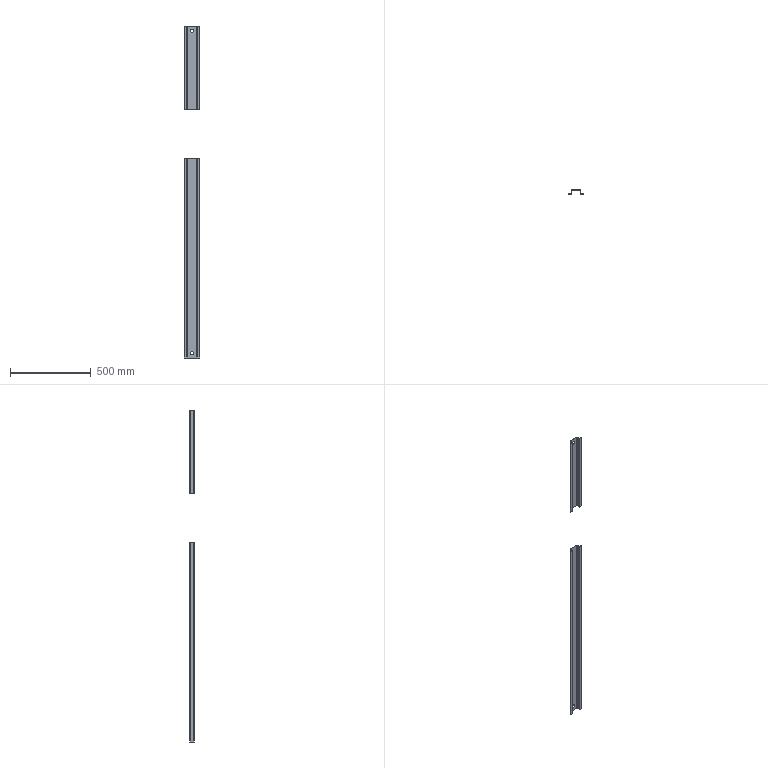Part | SolidWorks | features ICE 2, EdgeFlange 1, FlatPattern 1, SMBaseFlange 1, SheetMetal 1 | 2 solids | 80 faces | box 98.4 x 25 x 2051 mm | volume 201768 mm3 | plane 60 | cylinder 20 | commonest cylinder face diameters 2 x8 3.6 x8 20 x4